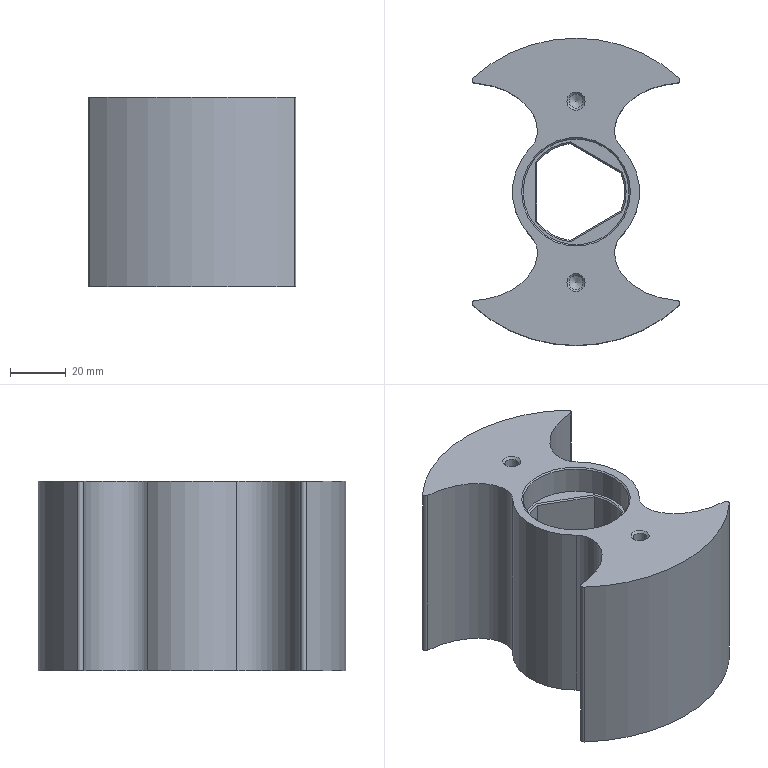Part | 1 solid | 50 faces | box 74.46 x 110.159 x 68 mm | volume 259040 mm3 | cylinder 17 | cone 16 | plane 13 | spline 4 | commonest cylinder face diameters 2.25 x4 35 x3 2.5 x2 5 x2 45.541 x2 110.159 x2
STEP:
#1=CARTESIAN_POINT('',(-1.35,20.25,-68.));
#2=VERTEX_POINT('',#1);
#3=CARTESIAN_POINT('',(0.,20.25,-68.));
#4=DIRECTION('',(0.,0.,-1.));
#5=DIRECTION('',(-1.,0.,0.));
#6=AXIS2_PLACEMENT_3D('',#3,#4,#5);
#7=CIRCLE('',#6,1.35);
#8=EDGE_CURVE('',#2,#2,#7,.T.);
#9=ORIENTED_EDGE('',*,*,#8,.F.);
#10=EDGE_LOOP('',(#9));
#11=FACE_BOUND('',#10,.T.);
#12=CARTESIAN_POINT('',(18.8,0.,-68.));
#13=VERTEX_POINT('',#12);
#14=CARTESIAN_POINT('',(0.,0.,-68.));
#15=DIRECTION('',(0.,0.,1.));
#16=DIRECTION('',(1.,0.,0.));
#17=AXIS2_PLACEMENT_3D('',#14,#15,#16);
#18=CIRCLE('',#17,18.8);
#19=EDGE_CURVE('',#13,#13,#18,.T.);
#20=ORIENTED_EDGE('',*,*,#19,.T.);
#21=EDGE_LOOP('',(#20));
#22=FACE_BOUND('',#21,.T.);
#23=CARTESIAN_POINT('',(-36.858,-40.93,-68.));
#24=VERTEX_POINT('',#23);
#25=CARTESIAN_POINT('',(36.858,-40.93,-68.));
#26=VERTEX_POINT('',#25);
#27=CARTESIAN_POINT('',(0.,0.,-68.));
#28=DIRECTION('',(0.,0.,1.));
#29=DIRECTION('',(1.,0.,0.));
#30=AXIS2_PLACEMENT_3D('',#27,#28,#29);
#31=CIRCLE('',#30,55.079);
#32=EDGE_CURVE('',#24,#26,#31,.T.);
#33=ORIENTED_EDGE('',*,*,#32,.F.);
#34=CARTESIAN_POINT('',(-36.188,-38.972,-68.));
#35=VERTEX_POINT('',#34);
#36=CARTESIAN_POINT('',(-36.105,-40.094,-68.));
#37=DIRECTION('',(0.,0.,1.));
#38=DIRECTION('',(1.,0.,0.));
#39=AXIS2_PLACEMENT_3D('',#36,#37,#38);
#40=CIRCLE('',#39,1.125);
#41=EDGE_CURVE('',#35,#24,#40,.T.);
#42=ORIENTED_EDGE('',*,*,#41,.F.);
#43=CARTESIAN_POINT('',(-16.101,-16.101,-68.));
#44=VERTEX_POINT('',#43);
#45=CARTESIAN_POINT('',(-16.101,-16.101,-68.));
#46=CARTESIAN_POINT('',(-14.995,-17.215,-68.));
#47=CARTESIAN_POINT('',(-13.563,-20.098,-68.));
#48=CARTESIAN_POINT('',(-13.933,-24.897,-68.));
#49=CARTESIAN_POINT('',(-16.007,-29.108,-68.));
#50=CARTESIAN_POINT('',(-20.192,-33.725,-68.));
#51=CARTESIAN_POINT('',(-27.057,-37.533,-68.));
#52=CARTESIAN_POINT('',(-33.099,-38.735,-68.));
#53=CARTESIAN_POINT('',(-36.188,-38.972,-68.));
#54=B_SPLINE_CURVE_WITH_KNOTS('',3,(#45,#46,#47,#48,#49,#50,#51,#52,#53),.UNSPECIFIED.,.F.,.F.,(4,1,1,1,1,1,4),(0.,0.004639,0.009278,0.01392,0.01856,0.02783,0.03711),.UNSPECIFIED.);
#55=EDGE_CURVE('',#44,#35,#54,.T.);
#56=ORIENTED_EDGE('',*,*,#55,.F.);
#57=CARTESIAN_POINT('',(-16.101,16.101,-68.));
#58=VERTEX_POINT('',#57);
#59=CARTESIAN_POINT('',(0.,0.,-68.));
#60=DIRECTION('',(0.,0.,1.));
#61=DIRECTION('',(1.,0.,0.));
#62=AXIS2_PLACEMENT_3D('',#59,#60,#61);
#63=CIRCLE('',#62,22.771);
#64=EDGE_CURVE('',#58,#44,#63,.T.);
#65=ORIENTED_EDGE('',*,*,#64,.F.);
#66=CARTESIAN_POINT('',(-36.188,38.972,-68.));
#67=VERTEX_POINT('',#66);
#68=CARTESIAN_POINT('',(-36.188,38.972,-68.));
#69=CARTESIAN_POINT('',(-33.1,38.735,-68.));
#70=CARTESIAN_POINT('',(-27.074,37.541,-68.));
#71=CARTESIAN_POINT('',(-20.182,33.717,-68.));
#72=CARTESIAN_POINT('',(-16.008,29.109,-68.));
#73=CARTESIAN_POINT('',(-13.931,24.889,-68.));
#74=CARTESIAN_POINT('',(-13.564,20.1,-68.));
#75=CARTESIAN_POINT('',(-14.995,17.216,-68.));
#76=CARTESIAN_POINT('',(-16.101,16.101,-68.));
#77=B_SPLINE_CURVE_WITH_KNOTS('',3,(#68,#69,#70,#71,#72,#73,#74,#75,#76),.UNSPECIFIED.,.F.,.F.,(4,1,1,1,1,1,4),(0.,0.009182,0.01836,0.02295,0.02755,0.03214,0.03673),.UNSPECIFIED.);
#78=EDGE_CURVE('',#67,#58,#77,.T.);
#79=ORIENTED_EDGE('',*,*,#78,.F.);
#80=CARTESIAN_POINT('',(-36.858,40.93,-68.));
#81=VERTEX_POINT('',#80);
#82=CARTESIAN_POINT('',(-36.105,40.094,-68.));
#83=DIRECTION('',(0.,0.,1.));
#84=DIRECTION('',(1.,0.,0.));
#85=AXIS2_PLACEMENT_3D('',#82,#83,#84);
#86=CIRCLE('',#85,1.125);
#87=EDGE_CURVE('',#81,#67,#86,.T.);
#88=ORIENTED_EDGE('',*,*,#87,.F.);
#89=CARTESIAN_POINT('',(36.858,40.93,-68.));
#90=VERTEX_POINT('',#89);
#91=CARTESIAN_POINT('',(0.,0.,-68.));
#92=DIRECTION('',(0.,0.,1.));
#93=DIRECTION('',(1.,0.,0.));
#94=AXIS2_PLACEMENT_3D('',#91,#92,#93);
#95=CIRCLE('',#94,55.079);
#96=EDGE_CURVE('',#90,#81,#95,.T.);
#97=ORIENTED_EDGE('',*,*,#96,.F.);
#98=CARTESIAN_POINT('',(36.188,38.972,-68.));
#99=VERTEX_POINT('',#98);
#100=CARTESIAN_POINT('',(36.105,40.094,-68.));
#101=DIRECTION('',(0.,0.,1.));
#102=DIRECTION('',(1.,0.,0.));
#103=AXIS2_PLACEMENT_3D('',#100,#101,#102);
#104=CIRCLE('',#103,1.125);
#105=EDGE_CURVE('',#99,#90,#104,.T.);
#106=ORIENTED_EDGE('',*,*,#105,.F.);
#107=CARTESIAN_POINT('',(16.101,16.101,-68.));
#108=VERTEX_POINT('',#107);
#109=CARTESIAN_POINT('',(16.101,16.101,-68.));
#110=CARTESIAN_POINT('',(14.995,17.215,-68.));
#111=CARTESIAN_POINT('',(13.563,20.098,-68.));
#112=CARTESIAN_POINT('',(13.933,24.897,-68.));
#113=CARTESIAN_POINT('',(16.007,29.108,-68.));
#114=CARTESIAN_POINT('',(20.192,33.725,-68.));
#115=CARTESIAN_POINT('',(27.057,37.533,-68.));
#116=CARTESIAN_POINT('',(33.099,38.735,-68.));
#117=CARTESIAN_POINT('',(36.188,38.972,-68.));
#118=B_SPLINE_CURVE_WITH_KNOTS('',3,(#109,#110,#111,#112,#113,#114,#115,#116,#117),.UNSPECIFIED.,.F.,.F.,(4,1,1,1,1,1,4),(0.,0.004639,0.009278,0.01392,0.01856,0.02783,0.03711),.UNSPECIFIED.);
#119=EDGE_CURVE('',#108,#99,#118,.T.);
#120=ORIENTED_EDGE('',*,*,#119,.F.);
#121=CARTESIAN_POINT('',(16.101,-16.101,-68.));
#122=VERTEX_POINT('',#121);
#123=CARTESIAN_POINT('',(0.,0.,-68.));
#124=DIRECTION('',(0.,0.,1.));
#125=DIRECTION('',(1.,0.,0.));
#126=AXIS2_PLACEMENT_3D('',#123,#124,#125);
#127=CIRCLE('',#126,22.771);
#128=EDGE_CURVE('',#122,#108,#127,.T.);
#129=ORIENTED_EDGE('',*,*,#128,.F.);
#130=CARTESIAN_POINT('',(36.188,-38.972,-68.));
#131=VERTEX_POINT('',#130);
#132=CARTESIAN_POINT('',(36.188,-38.972,-68.));
#133=CARTESIAN_POINT('',(33.1,-38.735,-68.));
#134=CARTESIAN_POINT('',(27.074,-37.541,-68.));
#135=CARTESIAN_POINT('',(20.182,-33.717,-68.));
#136=CARTESIAN_POINT('',(16.008,-29.109,-68.));
#137=CARTESIAN_POINT('',(13.931,-24.889,-68.));
#138=CARTESIAN_POINT('',(13.564,-20.1,-68.));
#139=CARTESIAN_POINT('',(14.995,-17.216,-68.));
#140=CARTESIAN_POINT('',(16.101,-16.101,-68.));
#141=B_SPLINE_CURVE_WITH_KNOTS('',3,(#132,#133,#134,#135,#136,#137,#138,#139,#140),.UNSPECIFIED.,.F.,.F.,(4,1,1,1,1,1,4),(0.,0.009182,0.01836,0.02295,0.02755,0.03214,0.03673),.UNSPECIFIED.);
#142=EDGE_CURVE('',#131,#122,#141,.T.);
#143=ORIENTED_EDGE('',*,*,#142,.F.);
#144=CARTESIAN_POINT('',(36.105,-40.094,-68.));
#145=DIRECTION('',(0.,0.,1.));
#146=DIRECTION('',(1.,0.,0.));
#147=AXIS2_PLACEMENT_3D('',#144,#145,#146);
#148=CIRCLE('',#147,1.125);
#149=EDGE_CURVE('',#26,#131,#148,.T.);
#150=ORIENTED_EDGE('',*,*,#149,.F.);
#151=EDGE_LOOP('',(#33,#42,#56,#65,#79,#88,#97,#106,#120,#129,#143,#150));
#152=FACE_BOUND('',#151,.T.);
#153=CARTESIAN_POINT('',(-1.35,-20.25,-68.));
#154=VERTEX_POINT('',#153);
#155=CARTESIAN_POINT('',(0.,-20.25,-68.));
#156=DIRECTION('',(0.,0.,-1.));
#157=DIRECTION('',(-1.,0.,0.));
#158=AXIS2_PLACEMENT_3D('',#155,#156,#157);
#159=CIRCLE('',#158,1.35);
#160=EDGE_CURVE('',#154,#154,#159,.T.);
#161=ORIENTED_EDGE('',*,*,#160,.F.);
#162=EDGE_LOOP('',(#161));
#163=FACE_BOUND('',#162,.T.);
#164=CARTESIAN_POINT('',(0.,0.,-68.));
#165=DIRECTION('',(0.,0.,1.));
#166=DIRECTION('',(1.,0.,0.));
#167=AXIS2_PLACEMENT_3D('',#164,#165,#166);
#168=PLANE('',#167);
#169=ADVANCED_FACE('',(#11,#22,#152,#163),#168,.F.);
#170=CARTESIAN_POINT('',(-2.093,17.374,-10.7));
#171=VERTEX_POINT('',#170);
#172=CARTESIAN_POINT('',(-2.093,17.374,-62.5));
#173=VERTEX_POINT('',#172);
#174=CARTESIAN_POINT('',(-2.093,17.374,11.09));
#175=DIRECTION('',(0.,0.,-1.));
#176=VECTOR('',#175,1000.);
#177=LINE('',#174,#176);
#178=EDGE_CURVE('',#171,#173,#177,.T.);
#179=ORIENTED_EDGE('',*,*,#178,.F.);
#180=CARTESIAN_POINT('',(-14.,10.5,-10.7));
#181=VERTEX_POINT('',#180);
#182=CARTESIAN_POINT('',(0.,0.,-10.7));
#183=DIRECTION('',(0.,0.,-1.));
#184=DIRECTION('',(-1.,0.,0.));
#185=AXIS2_PLACEMENT_3D('',#182,#183,#184);
#186=CIRCLE('',#185,17.5);
#187=EDGE_CURVE('',#171,#181,#186,.F.);
#188=ORIENTED_EDGE('',*,*,#187,.T.);
#189=CARTESIAN_POINT('',(-14.,10.5,-62.5));
#190=VERTEX_POINT('',#189);
#191=CARTESIAN_POINT('',(-14.,10.5,11.09));
#192=DIRECTION('',(0.,0.,-1.));
#193=VECTOR('',#192,1000.);
#194=LINE('',#191,#193);
#195=EDGE_CURVE('',#181,#190,#194,.T.);
#196=ORIENTED_EDGE('',*,*,#195,.T.);
#197=CARTESIAN_POINT('',(0.,0.,-62.5));
#198=DIRECTION('',(0.,0.,1.));
#199=DIRECTION('',(1.,0.,0.));
#200=AXIS2_PLACEMENT_3D('',#197,#198,#199);
#201=CIRCLE('',#200,17.5);
#202=EDGE_CURVE('',#190,#173,#201,.F.);
#203=ORIENTED_EDGE('',*,*,#202,.T.);
#204=EDGE_LOOP('',(#179,#188,#196,#203));
#205=FACE_BOUND('',#204,.T.);
#206=CARTESIAN_POINT('',(0.,0.,-68.));
#207=DIRECTION('',(0.,0.,-1.));
#208=DIRECTION('',(-1.,0.,0.));
#209=AXIS2_PLACEMENT_3D('',#206,#207,#208);
#210=CYLINDRICAL_SURFACE('',#209,17.5);
#211=ADVANCED_FACE('',(#205),#210,.F.);
#212=CARTESIAN_POINT('',(16.093,-6.874,-10.7));
#213=VERTEX_POINT('',#212);
#214=CARTESIAN_POINT('',(16.093,-6.874,-62.5));
#215=VERTEX_POINT('',#214);
#216=CARTESIAN_POINT('',(16.093,-6.874,11.09));
#217=DIRECTION('',(0.,0.,-1.));
#218=VECTOR('',#217,1000.);
#219=LINE('',#216,#218);
#220=EDGE_CURVE('',#213,#215,#219,.T.);
#221=ORIENTED_EDGE('',*,*,#220,.F.);
#222=CARTESIAN_POINT('',(16.093,6.874,-10.7));
#223=VERTEX_POINT('',#222);
#224=CARTESIAN_POINT('',(0.,0.,-10.7));
#225=DIRECTION('',(0.,0.,-1.));
#226=DIRECTION('',(-1.,0.,0.));
#227=AXIS2_PLACEMENT_3D('',#224,#225,#226);
#228=CIRCLE('',#227,17.5);
#229=EDGE_CURVE('',#213,#223,#228,.F.);
#230=ORIENTED_EDGE('',*,*,#229,.T.);
#231=CARTESIAN_POINT('',(16.093,6.874,-62.5));
#232=VERTEX_POINT('',#231);
#233=CARTESIAN_POINT('',(16.093,6.874,11.09));
#234=DIRECTION('',(0.,0.,-1.));
#235=VECTOR('',#234,1000.);
#236=LINE('',#233,#235);
#237=EDGE_CURVE('',#223,#232,#236,.T.);
#238=ORIENTED_EDGE('',*,*,#237,.T.);
#239=CARTESIAN_POINT('',(0.,0.,-62.5));
#240=DIRECTION('',(0.,0.,1.));
#241=DIRECTION('',(1.,0.,0.));
#242=AXIS2_PLACEMENT_3D('',#239,#240,#241);
#243=CIRCLE('',#242,17.5);
#244=EDGE_CURVE('',#232,#215,#243,.F.);
#245=ORIENTED_EDGE('',*,*,#244,.T.);
#246=EDGE_LOOP('',(#221,#230,#238,#245));
#247=FACE_BOUND('',#246,.T.);
#248=CARTESIAN_POINT('',(0.,0.,-68.));
#249=DIRECTION('',(0.,0.,-1.));
#250=DIRECTION('',(-1.,0.,0.));
#251=AXIS2_PLACEMENT_3D('',#248,#249,#250);
#252=CYLINDRICAL_SURFACE('',#251,17.5);
#253=ADVANCED_FACE('',(#247),#252,.F.);
#254=ORIENTED_EDGE('',*,*,#32,.T.);
#255=CARTESIAN_POINT('',(36.858,-40.93,0.));
#256=VERTEX_POINT('',#255);
#257=CARTESIAN_POINT('',(36.858,-40.93,0.));
#258=DIRECTION('',(0.,0.,-1.));
#259=VECTOR('',#258,1000.);
#260=LINE('',#257,#259);
#261=EDGE_CURVE('',#256,#26,#260,.T.);
#262=ORIENTED_EDGE('',*,*,#261,.F.);
#263=CARTESIAN_POINT('',(-36.858,-40.93,0.));
#264=VERTEX_POINT('',#263);
#265=CARTESIAN_POINT('',(0.,0.,0.));
#266=DIRECTION('',(0.,0.,1.));
#267=DIRECTION('',(1.,0.,0.));
#268=AXIS2_PLACEMENT_3D('',#265,#266,#267);
#269=CIRCLE('',#268,55.079);
#270=EDGE_CURVE('',#264,#256,#269,.T.);
#271=ORIENTED_EDGE('',*,*,#270,.F.);
#272=CARTESIAN_POINT('',(-36.858,-40.93,0.));
#273=DIRECTION('',(0.,0.,-1.));
#274=VECTOR('',#273,1000.);
#275=LINE('',#272,#274);
#276=EDGE_CURVE('',#264,#24,#275,.T.);
#277=ORIENTED_EDGE('',*,*,#276,.T.);
#278=EDGE_LOOP('',(#254,#262,#271,#277));
#279=FACE_BOUND('',#278,.T.);
#280=CARTESIAN_POINT('',(0.,0.,0.));
#281=DIRECTION('',(0.,0.,-1.));
#282=DIRECTION('',(-1.,0.,0.));
#283=AXIS2_PLACEMENT_3D('',#280,#281,#282);
#284=CYLINDRICAL_SURFACE('',#283,55.079);
#285=ADVANCED_FACE('',(#279),#284,.T.);
#286=ORIENTED_EDGE('',*,*,#149,.T.);
#287=CARTESIAN_POINT('',(36.188,-38.972,0.));
#288=VERTEX_POINT('',#287);
#289=CARTESIAN_POINT('',(36.188,-38.972,0.));
#290=DIRECTION('',(0.,0.,-1.));
#291=VECTOR('',#290,1000.);
#292=LINE('',#289,#291);
#293=EDGE_CURVE('',#288,#131,#292,.T.);
#294=ORIENTED_EDGE('',*,*,#293,.F.);
#295=CARTESIAN_POINT('',(36.105,-40.094,0.));
#296=DIRECTION('',(0.,0.,1.));
#297=DIRECTION('',(1.,0.,0.));
#298=AXIS2_PLACEMENT_3D('',#295,#296,#297);
#299=CIRCLE('',#298,1.125);
#300=EDGE_CURVE('',#256,#288,#299,.T.);
#301=ORIENTED_EDGE('',*,*,#300,.F.);
#302=ORIENTED_EDGE('',*,*,#261,.T.);
#303=EDGE_LOOP('',(#286,#294,#301,#302));
#304=FACE_BOUND('',#303,.T.);
#305=CARTESIAN_POINT('',(36.105,-40.094,0.));
#306=DIRECTION('',(0.,0.,-1.));
#307=DIRECTION('',(-1.,0.,0.));
#308=AXIS2_PLACEMENT_3D('',#305,#306,#307);
#309=CYLINDRICAL_SURFACE('',#308,1.125);
#310=ADVANCED_FACE('',(#304),#309,.T.);
#311=ORIENTED_EDGE('',*,*,#142,.T.);
#312=CARTESIAN_POINT('',(16.101,-16.101,0.));
#313=VERTEX_POINT('',#312);
#314=CARTESIAN_POINT('',(16.101,-16.101,0.));
#315=DIRECTION('',(0.,0.,-1.));
#316=VECTOR('',#315,1000.);
#317=LINE('',#314,#316);
#318=EDGE_CURVE('',#313,#122,#317,.T.);
#319=ORIENTED_EDGE('',*,*,#318,.F.);
#320=CARTESIAN_POINT('',(36.188,-38.972,0.));
#321=CARTESIAN_POINT('',(33.1,-38.735,0.));
#322=CARTESIAN_POINT('',(27.074,-37.541,0.));
#323=CARTESIAN_POINT('',(20.182,-33.717,0.));
#324=CARTESIAN_POINT('',(16.008,-29.109,0.));
#325=CARTESIAN_POINT('',(13.931,-24.889,0.));
#326=CARTESIAN_POINT('',(13.564,-20.1,0.));
#327=CARTESIAN_POINT('',(14.995,-17.216,0.));
#328=CARTESIAN_POINT('',(16.101,-16.101,0.));
#329=B_SPLINE_CURVE_WITH_KNOTS('',3,(#320,#321,#322,#323,#324,#325,#326,#327,#328),.UNSPECIFIED.,.F.,.F.,(4,1,1,1,1,1,4),(0.,0.009182,0.01836,0.02295,0.02755,0.03214,0.03673),.UNSPECIFIED.);
#330=EDGE_CURVE('',#288,#313,#329,.T.);
#331=ORIENTED_EDGE('',*,*,#330,.F.);
#332=ORIENTED_EDGE('',*,*,#293,.T.);
#333=EDGE_LOOP('',(#311,#319,#331,#332));
#334=FACE_BOUND('',#333,.T.);
#335=CARTESIAN_POINT('',(36.188,-38.972,0.));
#336=CARTESIAN_POINT('',(36.188,-38.972,-68.));
#337=CARTESIAN_POINT('',(33.121,-38.737,0.));
#338=CARTESIAN_POINT('',(33.121,-38.737,-68.));
#339=CARTESIAN_POINT('',(27.013,-37.524,0.));
#340=CARTESIAN_POINT('',(27.013,-37.524,-68.));
#341=CARTESIAN_POINT('',(20.163,-33.701,0.));
#342=CARTESIAN_POINT('',(20.163,-33.701,-68.));
#343=CARTESIAN_POINT('',(15.987,-29.082,0.));
#344=CARTESIAN_POINT('',(15.987,-29.082,-68.));
#345=CARTESIAN_POINT('',(13.93,-24.864,0.));
#346=CARTESIAN_POINT('',(13.93,-24.864,-68.));
#347=CARTESIAN_POINT('',(13.556,-20.109,0.));
#348=CARTESIAN_POINT('',(13.556,-20.109,-68.));
#349=CARTESIAN_POINT('',(15.018,-17.192,0.));
#350=CARTESIAN_POINT('',(15.018,-17.192,-68.));
#351=CARTESIAN_POINT('',(16.101,-16.101,0.));
#352=CARTESIAN_POINT('',(16.101,-16.101,-68.));
#353=B_SPLINE_SURFACE_WITH_KNOTS('',3,1,((#335,#336),(#337,#338),(#339,#340),(#341,#342),(#343,#344),(#345,#346),(#347,#348),(#349,#350),(#351,#352)),.SURF_OF_LINEAR_EXTRUSION.,.F.,.F.,.F.,(4,1,1,1,1,1,4),(2,2),(0.,0.25,0.5,0.625,0.75,0.875,1.),(0.,1.),.UNSPECIFIED.);
#354=ADVANCED_FACE('',(#334),#353,.F.);
#355=ORIENTED_EDGE('',*,*,#128,.T.);
#356=CARTESIAN_POINT('',(16.101,16.101,0.));
#357=VERTEX_POINT('',#356);
#358=CARTESIAN_POINT('',(16.101,16.101,0.));
#359=DIRECTION('',(0.,0.,-1.));
#360=VECTOR('',#359,1000.);
#361=LINE('',#358,#360);
#362=EDGE_CURVE('',#357,#108,#361,.T.);
#363=ORIENTED_EDGE('',*,*,#362,.F.);
#364=CARTESIAN_POINT('',(0.,0.,0.));
#365=DIRECTION('',(0.,0.,1.));
#366=DIRECTION('',(1.,0.,0.));
#367=AXIS2_PLACEMENT_3D('',#364,#365,#366);
#368=CIRCLE('',#367,22.771);
#369=EDGE_CURVE('',#313,#357,#368,.T.);
#370=ORIENTED_EDGE('',*,*,#369,.F.);
#371=ORIENTED_EDGE('',*,*,#318,.T.);
#372=EDGE_LOOP('',(#355,#363,#370,#371));
#373=FACE_BOUND('',#372,.T.);
#374=CARTESIAN_POINT('',(0.,0.,0.));
#375=DIRECTION('',(0.,0.,-1.));
#376=DIRECTION('',(-1.,0.,0.));
#377=AXIS2_PLACEMENT_3D('',#374,#375,#376);
#378=CYLINDRICAL_SURFACE('',#377,22.771);
#379=ADVANCED_FACE('',(#373),#378,.T.);
#380=ORIENTED_EDGE('',*,*,#119,.T.);
#381=CARTESIAN_POINT('',(36.188,38.972,0.));
#382=VERTEX_POINT('',#381);
#383=CARTESIAN_POINT('',(36.188,38.972,0.));
#384=DIRECTION('',(0.,0.,-1.));
#385=VECTOR('',#384,1000.);
#386=LINE('',#383,#385);
#387=EDGE_CURVE('',#382,#99,#386,.T.);
#388=ORIENTED_EDGE('',*,*,#387,.F.);
#389=CARTESIAN_POINT('',(16.101,16.101,0.));
#390=CARTESIAN_POINT('',(14.995,17.215,0.));
#391=CARTESIAN_POINT('',(13.563,20.098,0.));
#392=CARTESIAN_POINT('',(13.933,24.897,0.));
#393=CARTESIAN_POINT('',(16.007,29.108,0.));
#394=CARTESIAN_POINT('',(20.192,33.725,0.));
#395=CARTESIAN_POINT('',(27.057,37.533,0.));
#396=CARTESIAN_POINT('',(33.099,38.735,0.));
#397=CARTESIAN_POINT('',(36.188,38.972,0.));
#398=B_SPLINE_CURVE_WITH_KNOTS('',3,(#389,#390,#391,#392,#393,#394,#395,#396,#397),.UNSPECIFIED.,.F.,.F.,(4,1,1,1,1,1,4),(0.,0.004639,0.009278,0.01392,0.01856,0.02783,0.03711),.UNSPECIFIED.);
#399=EDGE_CURVE('',#357,#382,#398,.T.);
#400=ORIENTED_EDGE('',*,*,#399,.F.);
#401=ORIENTED_EDGE('',*,*,#362,.T.);
#402=EDGE_LOOP('',(#380,#388,#400,#401));
#403=FACE_BOUND('',#402,.T.);
#404=CARTESIAN_POINT('',(16.101,16.101,0.));
#405=CARTESIAN_POINT('',(16.101,16.101,-68.));
#406=CARTESIAN_POINT('',(15.018,17.192,0.));
#407=CARTESIAN_POINT('',(15.018,17.192,-68.));
#408=CARTESIAN_POINT('',(13.556,20.109,0.));
#409=CARTESIAN_POINT('',(13.556,20.109,-68.));
#410=CARTESIAN_POINT('',(13.93,24.864,0.));
#411=CARTESIAN_POINT('',(13.93,24.864,-68.));
#412=CARTESIAN_POINT('',(15.987,29.083,0.));
#413=CARTESIAN_POINT('',(15.987,29.083,-68.));
#414=CARTESIAN_POINT('',(20.163,33.702,0.));
#415=CARTESIAN_POINT('',(20.163,33.702,-68.));
#416=CARTESIAN_POINT('',(27.014,37.524,0.));
#417=CARTESIAN_POINT('',(27.014,37.524,-68.));
#418=CARTESIAN_POINT('',(33.122,38.737,0.));
#419=CARTESIAN_POINT('',(33.122,38.737,-68.));
#420=CARTESIAN_POINT('',(36.188,38.972,0.));
#421=CARTESIAN_POINT('',(36.188,38.972,-68.));
#422=B_SPLINE_SURFACE_WITH_KNOTS('',3,1,((#404,#405),(#406,#407),(#408,#409),(#410,#411),(#412,#413),(#414,#415),(#416,#417),(#418,#419),(#420,#421)),.SURF_OF_LINEAR_EXTRUSION.,.F.,.F.,.F.,(4,1,1,1,1,1,4),(2,2),(-0.000003449,0.125,0.25,0.375,0.5,0.75,1.),(0.,1.),.UNSPECIFIED.);
#423=ADVANCED_FACE('',(#403),#422,.F.);
#424=ORIENTED_EDGE('',*,*,#105,.T.);
#425=CARTESIAN_POINT('',(36.858,40.93,0.));
#426=VERTEX_POINT('',#425);
#427=CARTESIAN_POINT('',(36.858,40.93,0.));
#428=DIRECTION('',(0.,0.,-1.));
#429=VECTOR('',#428,1000.);
#430=LINE('',#427,#429);
#431=EDGE_CURVE('',#426,#90,#430,.T.);
#432=ORIENTED_EDGE('',*,*,#431,.F.);
#433=CARTESIAN_POINT('',(36.105,40.094,0.));
#434=DIRECTION('',(0.,0.,1.));
#435=DIRECTION('',(1.,0.,0.));
#436=AXIS2_PLACEMENT_3D('',#433,#434,#435);
#437=CIRCLE('',#436,1.125);
#438=EDGE_CURVE('',#382,#426,#437,.T.);
#439=ORIENTED_EDGE('',*,*,#438,.F.);
#440=ORIENTED_EDGE('',*,*,#387,.T.);
#441=EDGE_LOOP('',(#424,#432,#439,#440));
#442=FACE_BOUND('',#441,.T.);
#443=CARTESIAN_POINT('',(36.105,40.094,0.));
#444=DIRECTION('',(0.,0.,-1.));
#445=DIRECTION('',(-1.,0.,0.));
#446=AXIS2_PLACEMENT_3D('',#443,#444,#445);
#447=CYLINDRICAL_SURFACE('',#446,1.125);
#448=ADVANCED_FACE('',(#442),#447,.T.);
#449=ORIENTED_EDGE('',*,*,#96,.T.);
#450=CARTESIAN_POINT('',(-36.858,40.93,0.));
#451=VERTEX_POINT('',#450);
#452=CARTESIAN_POINT('',(-36.858,40.93,0.));
#453=DIRECTION('',(0.,0.,-1.));
#454=VECTOR('',#453,1000.);
#455=LINE('',#452,#454);
#456=EDGE_CURVE('',#451,#81,#455,.T.);
#457=ORIENTED_EDGE('',*,*,#456,.F.);
#458=CARTESIAN_POINT('',(0.,0.,0.));
#459=DIRECTION('',(0.,0.,1.));
#460=DIRECTION('',(1.,0.,0.));
#461=AXIS2_PLACEMENT_3D('',#458,#459,#460);
#462=CIRCLE('',#461,55.079);
#463=EDGE_CURVE('',#426,#451,#462,.T.);
#464=ORIENTED_EDGE('',*,*,#463,.F.);
#465=ORIENTED_EDGE('',*,*,#431,.T.);
#466=EDGE_LOOP('',(#449,#457,#464,#465));
#467=FACE_BOUND('',#466,.T.);
#468=CARTESIAN_POINT('',(0.,0.,0.));
#469=DIRECTION('',(0.,0.,-1.));
#470=DIRECTION('',(-1.,0.,0.));
#471=AXIS2_PLACEMENT_3D('',#468,#469,#470);
#472=CYLINDRICAL_SURFACE('',#471,55.079);
#473=ADVANCED_FACE('',(#467),#472,.T.);
#474=ORIENTED_EDGE('',*,*,#87,.T.);
#475=CARTESIAN_POINT('',(-36.188,38.972,0.));
#476=VERTEX_POINT('',#475);
#477=CARTESIAN_POINT('',(-36.188,38.972,0.));
#478=DIRECTION('',(0.,0.,-1.));
#479=VECTOR('',#478,1000.);
#480=LINE('',#477,#479);
#481=EDGE_CURVE('',#476,#67,#480,.T.);
#482=ORIENTED_EDGE('',*,*,#481,.F.);
#483=CARTESIAN_POINT('',(-36.105,40.094,0.));
#484=DIRECTION('',(0.,0.,1.));
#485=DIRECTION('',(1.,0.,0.));
#486=AXIS2_PLACEMENT_3D('',#483,#484,#485);
#487=CIRCLE('',#486,1.125);
#488=EDGE_CURVE('',#451,#476,#487,.T.);
#489=ORIENTED_EDGE('',*,*,#488,.F.);
#490=ORIENTED_EDGE('',*,*,#456,.T.);
#491=EDGE_LOOP('',(#474,#482,#489,#490));
#492=FACE_BOUND('',#491,.T.);
#493=CARTESIAN_POINT('',(-36.105,40.094,0.));
#494=DIRECTION('',(0.,0.,-1.));
#495=DIRECTION('',(-1.,0.,0.));
#496=AXIS2_PLACEMENT_3D('',#493,#494,#495);
#497=CYLINDRICAL_SURFACE('',#496,1.125);
#498=ADVANCED_FACE('',(#492),#497,.T.);
#499=ORIENTED_EDGE('',*,*,#78,.T.);
#500=CARTESIAN_POINT('',(-16.101,16.101,0.));
#501=VERTEX_POINT('',#500);
#502=CARTESIAN_POINT('',(-16.101,16.101,0.));
#503=DIRECTION('',(0.,0.,-1.));
#504=VECTOR('',#503,1000.);
#505=LINE('',#502,#504);
#506=EDGE_CURVE('',#501,#58,#505,.T.);
#507=ORIENTED_EDGE('',*,*,#506,.F.);
#508=CARTESIAN_POINT('',(-36.188,38.972,0.));
#509=CARTESIAN_POINT('',(-33.1,38.735,0.));
#510=CARTESIAN_POINT('',(-27.074,37.541,0.));
#511=CARTESIAN_POINT('',(-20.182,33.717,0.));
#512=CARTESIAN_POINT('',(-16.008,29.109,0.));
#513=CARTESIAN_POINT('',(-13.931,24.889,0.));
#514=CARTESIAN_POINT('',(-13.564,20.1,0.));
#515=CARTESIAN_POINT('',(-14.995,17.216,0.));
#516=CARTESIAN_POINT('',(-16.101,16.101,0.));
#517=B_SPLINE_CURVE_WITH_KNOTS('',3,(#508,#509,#510,#511,#512,#513,#514,#515,#516),.UNSPECIFIED.,.F.,.F.,(4,1,1,1,1,1,4),(0.,0.009182,0.01836,0.02295,0.02755,0.03214,0.03673),.UNSPECIFIED.);
#518=EDGE_CURVE('',#476,#501,#517,.T.);
#519=ORIENTED_EDGE('',*,*,#518,.F.);
#520=ORIENTED_EDGE('',*,*,#481,.T.);
#521=EDGE_LOOP('',(#499,#507,#519,#520));
#522=FACE_BOUND('',#521,.T.);
#523=CARTESIAN_POINT('',(-36.188,38.972,0.));
#524=CARTESIAN_POINT('',(-36.188,38.972,-68.));
#525=CARTESIAN_POINT('',(-33.121,38.737,0.));
#526=CARTESIAN_POINT('',(-33.121,38.737,-68.));
#527=CARTESIAN_POINT('',(-27.013,37.524,0.));
#528=CARTESIAN_POINT('',(-27.013,37.524,-68.));
#529=CARTESIAN_POINT('',(-20.163,33.701,0.));
#530=CARTESIAN_POINT('',(-20.163,33.701,-68.));
#531=CARTESIAN_POINT('',(-15.987,29.082,0.));
#532=CARTESIAN_POINT('',(-15.987,29.082,-68.));
#533=CARTESIAN_POINT('',(-13.93,24.864,0.));
#534=CARTESIAN_POINT('',(-13.93,24.864,-68.));
#535=CARTESIAN_POINT('',(-13.556,20.109,0.));
#536=CARTESIAN_POINT('',(-13.556,20.109,-68.));
#537=CARTESIAN_POINT('',(-15.018,17.192,0.));
#538=CARTESIAN_POINT('',(-15.018,17.192,-68.));
#539=CARTESIAN_POINT('',(-16.101,16.101,0.));
#540=CARTESIAN_POINT('',(-16.101,16.101,-68.));
#541=B_SPLINE_SURFACE_WITH_KNOTS('',3,1,((#523,#524),(#525,#526),(#527,#528),(#529,#530),(#531,#532),(#533,#534),(#535,#536),(#537,#538),(#539,#540)),.SURF_OF_LINEAR_EXTRUSION.,.F.,.F.,.F.,(4,1,1,1,1,1,4),(2,2),(0.,0.25,0.5,0.625,0.75,0.875,1.),(0.,1.),.UNSPECIFIED.);
#542=ADVANCED_FACE('',(#522),#541,.F.);
#543=ORIENTED_EDGE('',*,*,#64,.T.);
#544=CARTESIAN_POINT('',(-16.101,-16.101,0.));
#545=VERTEX_POINT('',#544);
#546=CARTESIAN_POINT('',(-16.101,-16.101,0.));
#547=DIRECTION('',(0.,0.,-1.));
#548=VECTOR('',#547,1000.);
#549=LINE('',#546,#548);
#550=EDGE_CURVE('',#545,#44,#549,.T.);
#551=ORIENTED_EDGE('',*,*,#550,.F.);
#552=CARTESIAN_POINT('',(0.,0.,0.));
#553=DIRECTION('',(0.,0.,1.));
#554=DIRECTION('',(1.,0.,0.));
#555=AXIS2_PLACEMENT_3D('',#552,#553,#554);
#556=CIRCLE('',#555,22.771);
#557=EDGE_CURVE('',#501,#545,#556,.T.);
#558=ORIENTED_EDGE('',*,*,#557,.F.);
#559=ORIENTED_EDGE('',*,*,#506,.T.);
#560=EDGE_LOOP('',(#543,#551,#558,#559));
#561=FACE_BOUND('',#560,.T.);
#562=CARTESIAN_POINT('',(0.,0.,0.));
#563=DIRECTION('',(0.,0.,-1.));
#564=DIRECTION('',(-1.,0.,0.));
#565=AXIS2_PLACEMENT_3D('',#562,#563,#564);
#566=CYLINDRICAL_SURFACE('',#565,22.771);
#567=ADVANCED_FACE('',(#561),#566,.T.);
#568=ORIENTED_EDGE('',*,*,#55,.T.);
#569=CARTESIAN_POINT('',(-36.188,-38.972,0.));
#570=VERTEX_POINT('',#569);
#571=CARTESIAN_POINT('',(-36.188,-38.972,0.));
#572=DIRECTION('',(0.,0.,-1.));
#573=VECTOR('',#572,1000.);
#574=LINE('',#571,#573);
#575=EDGE_CURVE('',#570,#35,#574,.T.);
#576=ORIENTED_EDGE('',*,*,#575,.F.);
#577=CARTESIAN_POINT('',(-16.101,-16.101,0.));
#578=CARTESIAN_POINT('',(-14.995,-17.215,0.));
#579=CARTESIAN_POINT('',(-13.563,-20.098,0.));
#580=CARTESIAN_POINT('',(-13.933,-24.897,0.));
#581=CARTESIAN_POINT('',(-16.007,-29.108,0.));
#582=CARTESIAN_POINT('',(-20.192,-33.725,0.));
#583=CARTESIAN_POINT('',(-27.057,-37.533,0.));
#584=CARTESIAN_POINT('',(-33.099,-38.735,0.));
#585=CARTESIAN_POINT('',(-36.188,-38.972,0.));
#586=B_SPLINE_CURVE_WITH_KNOTS('',3,(#577,#578,#579,#580,#581,#582,#583,#584,#585),.UNSPECIFIED.,.F.,.F.,(4,1,1,1,1,1,4),(0.,0.004639,0.009278,0.01392,0.01856,0.02783,0.03711),.UNSPECIFIED.);
#587=EDGE_CURVE('',#545,#570,#586,.T.);
#588=ORIENTED_EDGE('',*,*,#587,.F.);
#589=ORIENTED_EDGE('',*,*,#550,.T.);
#590=EDGE_LOOP('',(#568,#576,#588,#589));
#591=FACE_BOUND('',#590,.T.);
#592=CARTESIAN_POINT('',(-16.101,-16.101,0.));
#593=CARTESIAN_POINT('',(-16.101,-16.101,-68.));
#594=CARTESIAN_POINT('',(-15.018,-17.192,0.));
#595=CARTESIAN_POINT('',(-15.018,-17.192,-68.));
#596=CARTESIAN_POINT('',(-13.556,-20.109,0.));
#597=CARTESIAN_POINT('',(-13.556,-20.109,-68.));
#598=CARTESIAN_POINT('',(-13.93,-24.864,0.));
#599=CARTESIAN_POINT('',(-13.93,-24.864,-68.));
#600=CARTESIAN_POINT('',(-15.987,-29.083,0.));
#601=CARTESIAN_POINT('',(-15.987,-29.083,-68.));
#602=CARTESIAN_POINT('',(-20.163,-33.702,0.));
#603=CARTESIAN_POINT('',(-20.163,-33.702,-68.));
#604=CARTESIAN_POINT('',(-27.014,-37.524,0.));
#605=CARTESIAN_POINT('',(-27.014,-37.524,-68.));
#606=CARTESIAN_POINT('',(-33.122,-38.737,0.));
#607=CARTESIAN_POINT('',(-33.122,-38.737,-68.));
#608=CARTESIAN_POINT('',(-36.188,-38.972,0.));
#609=CARTESIAN_POINT('',(-36.188,-38.972,-68.));
#610=B_SPLINE_SURFACE_WITH_KNOTS('',3,1,((#592,#593),(#594,#595),(#596,#597),(#598,#599),(#600,#601),(#602,#603),(#604,#605),(#606,#607),(#608,#609)),.SURF_OF_LINEAR_EXTRUSION.,.F.,.F.,.F.,(4,1,1,1,1,1,4),(2,2),(-0.000003449,0.125,0.25,0.375,0.5,0.75,1.),(0.,1.),.UNSPECIFIED.);
#611=ADVANCED_FACE('',(#591),#610,.F.);
#612=ORIENTED_EDGE('',*,*,#41,.T.);
#613=ORIENTED_EDGE('',*,*,#276,.F.);
#614=CARTESIAN_POINT('',(-36.105,-40.094,0.));
#615=DIRECTION('',(0.,0.,1.));
#616=DIRECTION('',(1.,0.,0.));
#617=AXIS2_PLACEMENT_3D('',#614,#615,#616);
#618=CIRCLE('',#617,1.125);
#619=EDGE_CURVE('',#570,#264,#618,.T.);
#620=ORIENTED_EDGE('',*,*,#619,.F.);
#621=ORIENTED_EDGE('',*,*,#575,.T.);
#622=EDGE_LOOP('',(#612,#613,#620,#621));
#623=FACE_BOUND('',#622,.T.);
#624=CARTESIAN_POINT('',(-36.105,-40.094,0.));
#625=DIRECTION('',(0.,0.,-1.));
#626=DIRECTION('',(-1.,0.,0.));
#627=AXIS2_PLACEMENT_3D('',#624,#625,#626);
#628=CYLINDRICAL_SURFACE('',#627,1.125);
#629=ADVANCED_FACE('',(#623),#628,.T.);
#630=CARTESIAN_POINT('',(3.25,-32.5,0.));
#631=VERTEX_POINT('',#630);
#632=CARTESIAN_POINT('',(0.,-32.5,0.));
#633=DIRECTION('',(0.,0.,1.));
#634=DIRECTION('',(1.,0.,0.));
#635=AXIS2_PLACEMENT_3D('',#632,#633,#634);
#636=CIRCLE('',#635,3.25);
#637=EDGE_CURVE('',#631,#631,#636,.T.);
#638=ORIENTED_EDGE('',*,*,#637,.F.);
#639=EDGE_LOOP('',(#638));
#640=FACE_BOUND('',#639,.T.);
#641=CARTESIAN_POINT('',(3.25,32.5,0.));
#642=VERTEX_POINT('',#641);
#643=CARTESIAN_POINT('',(0.,32.5,0.));
#644=DIRECTION('',(0.,0.,1.));
#645=DIRECTION('',(1.,0.,0.));
#646=AXIS2_PLACEMENT_3D('',#643,#644,#645);
#647=CIRCLE('',#646,3.25);
#648=EDGE_CURVE('',#642,#642,#647,.T.);
#649=ORIENTED_EDGE('',*,*,#648,.F.);
#650=EDGE_LOOP('',(#649));
#651=FACE_BOUND('',#650,.T.);
#652=CARTESIAN_POINT('',(19.5,0.,0.));
#653=VERTEX_POINT('',#652);
#654=CARTESIAN_POINT('',(0.,0.,0.));
#655=DIRECTION('',(0.,0.,1.));
#656=DIRECTION('',(1.,0.,0.));
#657=AXIS2_PLACEMENT_3D('',#654,#655,#656);
#658=CIRCLE('',#657,19.5);
#659=EDGE_CURVE('',#653,#653,#658,.F.);
#660=ORIENTED_EDGE('',*,*,#659,.T.);
#661=EDGE_LOOP('',(#660));
#662=FACE_BOUND('',#661,.T.);
#663=ORIENTED_EDGE('',*,*,#270,.T.);
#664=ORIENTED_EDGE('',*,*,#300,.T.);
#665=ORIENTED_EDGE('',*,*,#330,.T.);
#666=ORIENTED_EDGE('',*,*,#369,.T.);
#667=ORIENTED_EDGE('',*,*,#399,.T.);
#668=ORIENTED_EDGE('',*,*,#438,.T.);
#669=ORIENTED_EDGE('',*,*,#463,.T.);
#670=ORIENTED_EDGE('',*,*,#488,.T.);
#671=ORIENTED_EDGE('',*,*,#518,.T.);
#672=ORIENTED_EDGE('',*,*,#557,.T.);
#673=ORIENTED_EDGE('',*,*,#587,.T.);
#674=ORIENTED_EDGE('',*,*,#619,.T.);
#675=EDGE_LOOP('',(#663,#664,#665,#666,#667,#668,#669,#670,#671,#672,#673,#674));
#676=FACE_BOUND('',#675,.T.);
#677=CARTESIAN_POINT('',(0.,0.,0.));
#678=DIRECTION('',(0.,0.,1.));
#679=DIRECTION('',(1.,0.,0.));
#680=AXIS2_PLACEMENT_3D('',#677,#678,#679);
#681=PLANE('',#680);
#682=ADVANCED_FACE('',(#640,#651,#662,#676),#681,.T.);
#683=CARTESIAN_POINT('',(19.,0.,-0.5));
#684=VERTEX_POINT('',#683);
#685=CARTESIAN_POINT('',(0.,0.,-0.5));
#686=DIRECTION('',(0.,0.,1.));
#687=DIRECTION('',(1.,0.,0.));
#688=AXIS2_PLACEMENT_3D('',#685,#686,#687);
#689=CIRCLE('',#688,19.);
#690=EDGE_CURVE('',#684,#684,#689,.T.);
#691=ORIENTED_EDGE('',*,*,#690,.T.);
#692=EDGE_LOOP('',(#691));
#693=FACE_BOUND('',#692,.T.);
#694=CARTESIAN_POINT('',(-19.,0.,-10.2));
#695=VERTEX_POINT('',#694);
#696=CARTESIAN_POINT('',(0.,0.,-10.2));
#697=DIRECTION('',(0.,0.,-1.));
#698=DIRECTION('',(-1.,0.,0.));
#699=AXIS2_PLACEMENT_3D('',#696,#697,#698);
#700=CIRCLE('',#699,19.);
#701=EDGE_CURVE('',#695,#695,#700,.T.);
#702=ORIENTED_EDGE('',*,*,#701,.T.);
#703=EDGE_LOOP('',(#702));
#704=FACE_BOUND('',#703,.T.);
#705=CARTESIAN_POINT('',(0.,0.,-68.));
#706=DIRECTION('',(0.,0.,-1.));
#707=DIRECTION('',(-1.,0.,0.));
#708=AXIS2_PLACEMENT_3D('',#705,#706,#707);
#709=CYLINDRICAL_SURFACE('',#708,19.);
#710=ADVANCED_FACE('',(#693,#704),#709,.F.);
#711=CARTESIAN_POINT('',(-1.986,-17.89,-10.2));
#712=VERTEX_POINT('',#711);
#713=CARTESIAN_POINT('',(-14.5,-10.665,-10.2));
#714=VERTEX_POINT('',#713);
#715=CARTESIAN_POINT('',(0.,0.,-10.2));
#716=DIRECTION('',(0.,0.,-1.));
#717=DIRECTION('',(-1.,0.,0.));
#718=AXIS2_PLACEMENT_3D('',#715,#716,#717);
#719=CIRCLE('',#718,18.);
#720=EDGE_CURVE('',#712,#714,#719,.T.);
#721=ORIENTED_EDGE('',*,*,#720,.T.);
#722=CARTESIAN_POINT('',(-14.5,10.665,-10.2));
#723=VERTEX_POINT('',#722);
#724=CARTESIAN_POINT('',(-14.5,10.5,-10.2));
#725=DIRECTION('',(0.,1.,0.));
#726=VECTOR('',#725,1000.);
#727=LINE('',#724,#726);
#728=EDGE_CURVE('',#714,#723,#727,.T.);
#729=ORIENTED_EDGE('',*,*,#728,.T.);
#730=CARTESIAN_POINT('',(-1.986,17.89,-10.2));
#731=VERTEX_POINT('',#730);
#732=CARTESIAN_POINT('',(0.,0.,-10.2));
#733=DIRECTION('',(0.,0.,-1.));
#734=DIRECTION('',(-1.,0.,0.));
#735=AXIS2_PLACEMENT_3D('',#732,#733,#734);
#736=CIRCLE('',#735,18.);
#737=EDGE_CURVE('',#723,#731,#736,.T.);
#738=ORIENTED_EDGE('',*,*,#737,.T.);
#739=CARTESIAN_POINT('',(16.486,7.225,-10.2));
#740=VERTEX_POINT('',#739);
#741=CARTESIAN_POINT('',(16.343,7.307,-10.2));
#742=DIRECTION('',(0.866,-0.5,0.));
#743=VECTOR('',#742,1000.);
#744=LINE('',#741,#743);
#745=EDGE_CURVE('',#731,#740,#744,.T.);
#746=ORIENTED_EDGE('',*,*,#745,.T.);
#747=CARTESIAN_POINT('',(16.486,-7.225,-10.2));
#748=VERTEX_POINT('',#747);
#749=CARTESIAN_POINT('',(0.,0.,-10.2));
#750=DIRECTION('',(0.,0.,-1.));
#751=DIRECTION('',(-1.,0.,0.));
#752=AXIS2_PLACEMENT_3D('',#749,#750,#751);
#753=CIRCLE('',#752,18.);
#754=EDGE_CURVE('',#740,#748,#753,.T.);
#755=ORIENTED_EDGE('',*,*,#754,.T.);
#756=CARTESIAN_POINT('',(-1.843,-17.807,-10.2));
#757=DIRECTION('',(-0.866,-0.5,0.));
#758=VECTOR('',#757,1000.);
#759=LINE('',#756,#758);
#760=EDGE_CURVE('',#748,#712,#759,.T.);
#761=ORIENTED_EDGE('',*,*,#760,.T.);
#762=EDGE_LOOP('',(#721,#729,#738,#746,#755,#761));
#763=FACE_BOUND('',#762,.T.);
#764=ORIENTED_EDGE('',*,*,#701,.F.);
#765=EDGE_LOOP('',(#764));
#766=FACE_BOUND('',#765,.T.);
#767=CARTESIAN_POINT('',(0.,19.,-10.2));
#768=DIRECTION('',(0.,0.,-1.));
#769=DIRECTION('',(-1.,0.,0.));
#770=AXIS2_PLACEMENT_3D('',#767,#768,#769);
#771=PLANE('',#770);
#772=ADVANCED_FACE('',(#763,#766),#771,.F.);
#773=CARTESIAN_POINT('',(-14.,-10.5,-10.7));
#774=VERTEX_POINT('',#773);
#775=CARTESIAN_POINT('',(-14.,-10.5,-62.5));
#776=VERTEX_POINT('',#775);
#777=CARTESIAN_POINT('',(-14.,-10.5,11.09));
#778=DIRECTION('',(0.,0.,-1.));
#779=VECTOR('',#778,1000.);
#780=LINE('',#777,#779);
#781=EDGE_CURVE('',#774,#776,#780,.T.);
#782=ORIENTED_EDGE('',*,*,#781,.F.);
#783=CARTESIAN_POINT('',(-2.093,-17.374,-10.7));
#784=VERTEX_POINT('',#783);
#785=CARTESIAN_POINT('',(0.,0.,-10.7));
#786=DIRECTION('',(0.,0.,-1.));
#787=DIRECTION('',(-1.,0.,0.));
#788=AXIS2_PLACEMENT_3D('',#785,#786,#787);
#789=CIRCLE('',#788,17.5);
#790=EDGE_CURVE('',#774,#784,#789,.F.);
#791=ORIENTED_EDGE('',*,*,#790,.T.);
#792=CARTESIAN_POINT('',(-2.093,-17.374,-62.5));
#793=VERTEX_POINT('',#792);
#794=CARTESIAN_POINT('',(-2.093,-17.374,11.09));
#795=DIRECTION('',(0.,0.,-1.));
#796=VECTOR('',#795,1000.);
#797=LINE('',#794,#796);
#798=EDGE_CURVE('',#784,#793,#797,.T.);
#799=ORIENTED_EDGE('',*,*,#798,.T.);
#800=CARTESIAN_POINT('',(0.,0.,-62.5));
#801=DIRECTION('',(0.,0.,1.));
#802=DIRECTION('',(1.,0.,0.));
#803=AXIS2_PLACEMENT_3D('',#800,#801,#802);
#804=CIRCLE('',#803,17.5);
#805=EDGE_CURVE('',#793,#776,#804,.F.);
#806=ORIENTED_EDGE('',*,*,#805,.T.);
#807=EDGE_LOOP('',(#782,#791,#799,#806));
#808=FACE_BOUND('',#807,.T.);
#809=CARTESIAN_POINT('',(0.,0.,-68.));
#810=DIRECTION('',(0.,0.,-1.));
#811=DIRECTION('',(-1.,0.,0.));
#812=AXIS2_PLACEMENT_3D('',#809,#810,#811);
#813=CYLINDRICAL_SURFACE('',#812,17.5);
#814=ADVANCED_FACE('',(#808),#813,.F.);
#815=CARTESIAN_POINT('',(16.486,7.225,-63.));
#816=VERTEX_POINT('',#815);
#817=CARTESIAN_POINT('',(-1.986,17.89,-63.));
#818=VERTEX_POINT('',#817);
#819=CARTESIAN_POINT('',(-1.843,17.807,-63.));
#820=DIRECTION('',(-0.866,0.5,0.));
#821=VECTOR('',#820,1000.);
#822=LINE('',#819,#821);
#823=EDGE_CURVE('',#816,#818,#822,.T.);
#824=ORIENTED_EDGE('',*,*,#823,.T.);
#825=CARTESIAN_POINT('',(-14.5,10.665,-63.));
#826=VERTEX_POINT('',#825);
#827=CARTESIAN_POINT('',(0.,0.,-63.));
#828=DIRECTION('',(0.,0.,1.));
#829=DIRECTION('',(1.,0.,0.));
#830=AXIS2_PLACEMENT_3D('',#827,#828,#829);
#831=CIRCLE('',#830,18.);
#832=EDGE_CURVE('',#818,#826,#831,.T.);
#833=ORIENTED_EDGE('',*,*,#832,.T.);
#834=CARTESIAN_POINT('',(-14.5,-10.665,-63.));
#835=VERTEX_POINT('',#834);
#836=CARTESIAN_POINT('',(-14.5,-10.5,-63.));
#837=DIRECTION('',(0.,-1.,0.));
#838=VECTOR('',#837,1000.);
#839=LINE('',#836,#838);
#840=EDGE_CURVE('',#826,#835,#839,.T.);
#841=ORIENTED_EDGE('',*,*,#840,.T.);
#842=CARTESIAN_POINT('',(-1.986,-17.89,-63.));
#843=VERTEX_POINT('',#842);
#844=CARTESIAN_POINT('',(0.,0.,-63.));
#845=DIRECTION('',(0.,0.,1.));
#846=DIRECTION('',(1.,0.,0.));
#847=AXIS2_PLACEMENT_3D('',#844,#845,#846);
#848=CIRCLE('',#847,18.);
#849=EDGE_CURVE('',#835,#843,#848,.T.);
#850=ORIENTED_EDGE('',*,*,#849,.T.);
#851=CARTESIAN_POINT('',(16.486,-7.225,-63.));
#852=VERTEX_POINT('',#851);
#853=CARTESIAN_POINT('',(16.343,-7.307,-63.));
#854=DIRECTION('',(0.866,0.5,0.));
#855=VECTOR('',#854,1000.);
#856=LINE('',#853,#855);
#857=EDGE_CURVE('',#843,#852,#856,.T.);
#858=ORIENTED_EDGE('',*,*,#857,.T.);
#859=CARTESIAN_POINT('',(0.,0.,-63.));
#860=DIRECTION('',(0.,0.,1.));
#861=DIRECTION('',(1.,0.,0.));
#862=AXIS2_PLACEMENT_3D('',#859,#860,#861);
#863=CIRCLE('',#862,18.);
#864=EDGE_CURVE('',#852,#816,#863,.T.);
#865=ORIENTED_EDGE('',*,*,#864,.T.);
#866=EDGE_LOOP('',(#824,#833,#841,#850,#858,#865));
#867=FACE_BOUND('',#866,.T.);
#868=CARTESIAN_POINT('',(-18.3,0.,-63.));
#869=VERTEX_POINT('',#868);
#870=CARTESIAN_POINT('',(0.,0.,-63.));
#871=DIRECTION('',(0.,0.,-1.));
#872=DIRECTION('',(-1.,0.,0.));
#873=AXIS2_PLACEMENT_3D('',#870,#871,#872);
#874=CIRCLE('',#873,18.3);
#875=EDGE_CURVE('',#869,#869,#874,.T.);
#876=ORIENTED_EDGE('',*,*,#875,.T.);
#877=EDGE_LOOP('',(#876));
#878=FACE_BOUND('',#877,.T.);
#879=CARTESIAN_POINT('',(0.,17.5,-63.));
#880=DIRECTION('',(0.,0.,1.));
#881=DIRECTION('',(1.,0.,0.));
#882=AXIS2_PLACEMENT_3D('',#879,#880,#881);
#883=PLANE('',#882);
#884=ADVANCED_FACE('',(#867,#878),#883,.F.);
#885=CARTESIAN_POINT('',(18.3,0.,-67.5));
#886=VERTEX_POINT('',#885);
#887=CARTESIAN_POINT('',(0.,0.,-67.5));
#888=DIRECTION('',(0.,0.,1.));
#889=DIRECTION('',(1.,0.,0.));
#890=AXIS2_PLACEMENT_3D('',#887,#888,#889);
#891=CIRCLE('',#890,18.3);
#892=EDGE_CURVE('',#886,#886,#891,.F.);
#893=ORIENTED_EDGE('',*,*,#892,.T.);
#894=EDGE_LOOP('',(#893));
#895=FACE_BOUND('',#894,.T.);
#896=ORIENTED_EDGE('',*,*,#875,.F.);
#897=EDGE_LOOP('',(#896));
#898=FACE_BOUND('',#897,.T.);
#899=CARTESIAN_POINT('',(0.,0.,-68.));
#900=DIRECTION('',(0.,0.,-1.));
#901=DIRECTION('',(-1.,0.,0.));
#902=AXIS2_PLACEMENT_3D('',#899,#900,#901);
#903=CYLINDRICAL_SURFACE('',#902,18.3);
#904=ADVANCED_FACE('',(#895,#898),#903,.F.);
#905=ORIENTED_EDGE('',*,*,#195,.F.);
#906=CARTESIAN_POINT('',(-14.,-10.5,-10.7));
#907=DIRECTION('',(0.,-1.,0.));
#908=VECTOR('',#907,1000.);
#909=LINE('',#906,#908);
#910=EDGE_CURVE('',#181,#774,#909,.T.);
#911=ORIENTED_EDGE('',*,*,#910,.T.);
#912=ORIENTED_EDGE('',*,*,#781,.T.);
#913=CARTESIAN_POINT('',(-14.,10.5,-62.5));
#914=DIRECTION('',(0.,1.,0.));
#915=VECTOR('',#914,1000.);
#916=LINE('',#913,#915);
#917=EDGE_CURVE('',#776,#190,#916,.T.);
#918=ORIENTED_EDGE('',*,*,#917,.T.);
#919=EDGE_LOOP('',(#905,#911,#912,#918));
#920=FACE_BOUND('',#919,.T.);
#921=CARTESIAN_POINT('',(-14.,-10.5,11.09));
#922=DIRECTION('',(1.,0.,0.));
#923=DIRECTION('',(0.,0.,-1.));
#924=AXIS2_PLACEMENT_3D('',#921,#922,#923);
#925=PLANE('',#924);
#926=ADVANCED_FACE('',(#920),#925,.T.);
#927=ORIENTED_EDGE('',*,*,#798,.F.);
#928=CARTESIAN_POINT('',(16.093,-6.874,-10.7));
#929=DIRECTION('',(0.866,0.5,0.));
#930=VECTOR('',#929,1000.);
#931=LINE('',#928,#930);
#932=EDGE_CURVE('',#784,#213,#931,.T.);
#933=ORIENTED_EDGE('',*,*,#932,.T.);
#934=ORIENTED_EDGE('',*,*,#220,.T.);
#935=CARTESIAN_POINT('',(-2.093,-17.374,-62.5));
#936=DIRECTION('',(-0.866,-0.5,0.));
#937=VECTOR('',#936,1000.);
#938=LINE('',#935,#937);
#939=EDGE_CURVE('',#215,#793,#938,.T.);
#940=ORIENTED_EDGE('',*,*,#939,.T.);
#941=EDGE_LOOP('',(#927,#933,#934,#940));
#942=FACE_BOUND('',#941,.T.);
#943=CARTESIAN_POINT('',(16.093,-6.874,11.09));
#944=DIRECTION('',(-0.5,0.866,0.));
#945=DIRECTION('',(-0.866,-0.5,0.));
#946=AXIS2_PLACEMENT_3D('',#943,#944,#945);
#947=PLANE('',#946);
#948=ADVANCED_FACE('',(#942),#947,.T.);
#949=ORIENTED_EDGE('',*,*,#237,.F.);
#950=CARTESIAN_POINT('',(-2.093,17.374,-10.7));
#951=DIRECTION('',(-0.866,0.5,0.));
#952=VECTOR('',#951,1000.);
#953=LINE('',#950,#952);
#954=EDGE_CURVE('',#223,#171,#953,.T.);
#955=ORIENTED_EDGE('',*,*,#954,.T.);
#956=ORIENTED_EDGE('',*,*,#178,.T.);
#957=CARTESIAN_POINT('',(16.093,6.874,-62.5));
#958=DIRECTION('',(0.866,-0.5,0.));
#959=VECTOR('',#958,1000.);
#960=LINE('',#957,#959);
#961=EDGE_CURVE('',#173,#232,#960,.T.);
#962=ORIENTED_EDGE('',*,*,#961,.T.);
#963=EDGE_LOOP('',(#949,#955,#956,#962));
#964=FACE_BOUND('',#963,.T.);
#965=CARTESIAN_POINT('',(-2.093,17.374,11.09));
#966=DIRECTION('',(-0.5,-0.866,0.));
#967=DIRECTION('',(0.866,-0.5,0.));
#968=AXIS2_PLACEMENT_3D('',#965,#966,#967);
#969=PLANE('',#968);
#970=ADVANCED_FACE('',(#964),#969,.T.);
#971=CARTESIAN_POINT('',(16.486,7.225,-10.2));
#972=CARTESIAN_POINT('',(16.356,7.108,-10.367));
#973=CARTESIAN_POINT('',(16.225,6.991,-10.533));
#974=CARTESIAN_POINT('',(16.093,6.874,-10.7));
#975=B_SPLINE_CURVE_WITH_KNOTS('',3,(#971,#972,#973,#974),.UNSPECIFIED.,.F.,.F.,(4,4),(0.,0.0007262),.UNSPECIFIED.);
#976=EDGE_CURVE('',#223,#740,#975,.F.);
#977=ORIENTED_EDGE('',*,*,#976,.F.);
#978=ORIENTED_EDGE('',*,*,#229,.F.);
#979=CARTESIAN_POINT('',(16.486,-7.225,-10.2));
#980=CARTESIAN_POINT('',(16.356,-7.108,-10.367));
#981=CARTESIAN_POINT('',(16.225,-6.991,-10.533));
#982=CARTESIAN_POINT('',(16.093,-6.874,-10.7));
#983=B_SPLINE_CURVE_WITH_KNOTS('',3,(#979,#980,#981,#982),.UNSPECIFIED.,.F.,.F.,(4,4),(0.,0.0007262),.UNSPECIFIED.);
#984=EDGE_CURVE('',#748,#213,#983,.T.);
#985=ORIENTED_EDGE('',*,*,#984,.F.);
#986=ORIENTED_EDGE('',*,*,#754,.F.);
#987=EDGE_LOOP('',(#977,#978,#985,#986));
#988=FACE_BOUND('',#987,.T.);
#989=CARTESIAN_POINT('',(0.,0.,-10.2));
#990=DIRECTION('',(0.,0.,1.));
#991=DIRECTION('',(1.,0.,0.));
#992=AXIS2_PLACEMENT_3D('',#989,#990,#991);
#993=CONICAL_SURFACE('',#992,18.,0.7854);
#994=ADVANCED_FACE('',(#988),#993,.F.);
#995=ORIENTED_EDGE('',*,*,#984,.T.);
#996=ORIENTED_EDGE('',*,*,#932,.F.);
#997=CARTESIAN_POINT('',(-1.986,-17.89,-10.2));
#998=CARTESIAN_POINT('',(-2.022,-17.718,-10.367));
#999=CARTESIAN_POINT('',(-2.058,-17.546,-10.533));
#1000=CARTESIAN_POINT('',(-2.093,-17.374,-10.7));
#1001=B_SPLINE_CURVE_WITH_KNOTS('',3,(#997,#998,#999,#1000),.UNSPECIFIED.,.F.,.F.,(4,4),(0.,0.0007262),.UNSPECIFIED.);
#1002=EDGE_CURVE('',#712,#784,#1001,.T.);
#1003=ORIENTED_EDGE('',*,*,#1002,.F.);
#1004=ORIENTED_EDGE('',*,*,#760,.F.);
#1005=EDGE_LOOP('',(#995,#996,#1003,#1004));
#1006=FACE_BOUND('',#1005,.T.);
#1007=CARTESIAN_POINT('',(15.477,-7.807,-10.2));
#1008=DIRECTION('',(-0.3536,0.6124,0.7071));
#1009=DIRECTION('',(0.866,0.5,0.));
#1010=AXIS2_PLACEMENT_3D('',#1007,#1008,#1009);
#1011=PLANE('',#1010);
#1012=ADVANCED_FACE('',(#1006),#1011,.T.);
#1013=ORIENTED_EDGE('',*,*,#976,.T.);
#1014=ORIENTED_EDGE('',*,*,#745,.F.);
#1015=CARTESIAN_POINT('',(-1.986,17.89,-10.2));
#1016=CARTESIAN_POINT('',(-2.022,17.718,-10.367));
#1017=CARTESIAN_POINT('',(-2.058,17.546,-10.533));
#1018=CARTESIAN_POINT('',(-2.093,17.374,-10.7));
#1019=B_SPLINE_CURVE_WITH_KNOTS('',3,(#1015,#1016,#1017,#1018),.UNSPECIFIED.,.F.,.F.,(4,4),(0.,0.0007262),.UNSPECIFIED.);
#1020=EDGE_CURVE('',#171,#731,#1019,.F.);
#1021=ORIENTED_EDGE('',*,*,#1020,.F.);
#1022=ORIENTED_EDGE('',*,*,#954,.F.);
#1023=EDGE_LOOP('',(#1013,#1014,#1021,#1022));
#1024=FACE_BOUND('',#1023,.T.);
#1025=CARTESIAN_POINT('',(-0.9772,17.307,-10.2));
#1026=DIRECTION('',(-0.3536,-0.6124,0.7071));
#1027=DIRECTION('',(-0.866,0.5,0.));
#1028=AXIS2_PLACEMENT_3D('',#1025,#1026,#1027);
#1029=PLANE('',#1028);
#1030=ADVANCED_FACE('',(#1024),#1029,.T.);
#1031=ORIENTED_EDGE('',*,*,#1002,.T.);
#1032=ORIENTED_EDGE('',*,*,#790,.F.);
#1033=CARTESIAN_POINT('',(-14.,-10.5,-10.7));
#1034=CARTESIAN_POINT('',(-14.167,-10.556,-10.533));
#1035=CARTESIAN_POINT('',(-14.333,-10.611,-10.367));
#1036=CARTESIAN_POINT('',(-14.5,-10.665,-10.2));
#1037=B_SPLINE_CURVE_WITH_KNOTS('',3,(#1033,#1034,#1035,#1036),.UNSPECIFIED.,.F.,.F.,(4,4),(0.,0.0007262),.UNSPECIFIED.);
#1038=EDGE_CURVE('',#714,#774,#1037,.F.);
#1039=ORIENTED_EDGE('',*,*,#1038,.F.);
#1040=ORIENTED_EDGE('',*,*,#720,.F.);
#1041=EDGE_LOOP('',(#1031,#1032,#1039,#1040));
#1042=FACE_BOUND('',#1041,.T.);
#1043=CARTESIAN_POINT('',(0.,0.,-10.2));
#1044=DIRECTION('',(0.,0.,1.));
#1045=DIRECTION('',(1.,0.,0.));
#1046=AXIS2_PLACEMENT_3D('',#1043,#1044,#1045);
#1047=CONICAL_SURFACE('',#1046,18.,0.7854);
#1048=ADVANCED_FACE('',(#1042),#1047,.F.);
#1049=ORIENTED_EDGE('',*,*,#1020,.T.);
#1050=ORIENTED_EDGE('',*,*,#737,.F.);
#1051=CARTESIAN_POINT('',(-14.5,10.665,-10.2));
#1052=CARTESIAN_POINT('',(-14.333,10.611,-10.367));
#1053=CARTESIAN_POINT('',(-14.167,10.556,-10.533));
#1054=CARTESIAN_POINT('',(-14.,10.5,-10.7));
#1055=B_SPLINE_CURVE_WITH_KNOTS('',3,(#1051,#1052,#1053,#1054),.UNSPECIFIED.,.F.,.F.,(4,4),(0.,0.0007262),.UNSPECIFIED.);
#1056=EDGE_CURVE('',#181,#723,#1055,.F.);
#1057=ORIENTED_EDGE('',*,*,#1056,.F.);
#1058=ORIENTED_EDGE('',*,*,#187,.F.);
#1059=EDGE_LOOP('',(#1049,#1050,#1057,#1058));
#1060=FACE_BOUND('',#1059,.T.);
#1061=CARTESIAN_POINT('',(0.,0.,-10.2));
#1062=DIRECTION('',(0.,0.,1.));
#1063=DIRECTION('',(1.,0.,0.));
#1064=AXIS2_PLACEMENT_3D('',#1061,#1062,#1063);
#1065=CONICAL_SURFACE('',#1064,18.,0.7854);
#1066=ADVANCED_FACE('',(#1060),#1065,.F.);
#1067=ORIENTED_EDGE('',*,*,#1038,.T.);
#1068=ORIENTED_EDGE('',*,*,#910,.F.);
#1069=ORIENTED_EDGE('',*,*,#1056,.T.);
#1070=ORIENTED_EDGE('',*,*,#728,.F.);
#1071=EDGE_LOOP('',(#1067,#1068,#1069,#1070));
#1072=FACE_BOUND('',#1071,.T.);
#1073=CARTESIAN_POINT('',(-14.5,19.,-10.2));
#1074=DIRECTION('',(0.7071,0.,0.7071));
#1075=DIRECTION('',(0.,-1.,0.));
#1076=AXIS2_PLACEMENT_3D('',#1073,#1074,#1075);
#1077=PLANE('',#1076);
#1078=ADVANCED_FACE('',(#1072),#1077,.T.);
#1079=CARTESIAN_POINT('',(16.486,-7.225,-63.));
#1080=CARTESIAN_POINT('',(16.356,-7.108,-62.833));
#1081=CARTESIAN_POINT('',(16.225,-6.991,-62.667));
#1082=CARTESIAN_POINT('',(16.093,-6.874,-62.5));
#1083=B_SPLINE_CURVE_WITH_KNOTS('',3,(#1079,#1080,#1081,#1082),.UNSPECIFIED.,.F.,.F.,(4,4),(0.,0.0007262),.UNSPECIFIED.);
#1084=EDGE_CURVE('',#852,#215,#1083,.T.);
#1085=ORIENTED_EDGE('',*,*,#1084,.F.);
#1086=ORIENTED_EDGE('',*,*,#857,.F.);
#1087=CARTESIAN_POINT('',(-1.986,-17.89,-63.));
#1088=CARTESIAN_POINT('',(-2.022,-17.718,-62.833));
#1089=CARTESIAN_POINT('',(-2.058,-17.546,-62.667));
#1090=CARTESIAN_POINT('',(-2.093,-17.374,-62.5));
#1091=B_SPLINE_CURVE_WITH_KNOTS('',3,(#1087,#1088,#1089,#1090),.UNSPECIFIED.,.F.,.F.,(4,4),(0.,0.0007262),.UNSPECIFIED.);
#1092=EDGE_CURVE('',#793,#843,#1091,.F.);
#1093=ORIENTED_EDGE('',*,*,#1092,.F.);
#1094=ORIENTED_EDGE('',*,*,#939,.F.);
#1095=EDGE_LOOP('',(#1085,#1086,#1093,#1094));
#1096=FACE_BOUND('',#1095,.T.);
#1097=CARTESIAN_POINT('',(14.828,-8.182,-63.));
#1098=DIRECTION('',(-0.3536,0.6124,-0.7071));
#1099=DIRECTION('',(-0.866,-0.5,0.));
#1100=AXIS2_PLACEMENT_3D('',#1097,#1098,#1099);
#1101=PLANE('',#1100);
#1102=ADVANCED_FACE('',(#1096),#1101,.T.);
#1103=ORIENTED_EDGE('',*,*,#1092,.T.);
#1104=ORIENTED_EDGE('',*,*,#849,.F.);
#1105=CARTESIAN_POINT('',(-14.5,-10.665,-63.));
#1106=CARTESIAN_POINT('',(-14.333,-10.611,-62.833));
#1107=CARTESIAN_POINT('',(-14.167,-10.556,-62.667));
#1108=CARTESIAN_POINT('',(-14.,-10.5,-62.5));
#1109=B_SPLINE_CURVE_WITH_KNOTS('',3,(#1105,#1106,#1107,#1108),.UNSPECIFIED.,.F.,.F.,(4,4),(0.,0.0007262),.UNSPECIFIED.);
#1110=EDGE_CURVE('',#776,#835,#1109,.F.);
#1111=ORIENTED_EDGE('',*,*,#1110,.F.);
#1112=ORIENTED_EDGE('',*,*,#805,.F.);
#1113=EDGE_LOOP('',(#1103,#1104,#1111,#1112));
#1114=FACE_BOUND('',#1113,.T.);
#1115=CARTESIAN_POINT('',(0.,0.,-62.5));
#1116=DIRECTION('',(0.,0.,-1.));
#1117=DIRECTION('',(-1.,0.,0.));
#1118=AXIS2_PLACEMENT_3D('',#1115,#1116,#1117);
#1119=CONICAL_SURFACE('',#1118,17.5,0.7854);
#1120=ADVANCED_FACE('',(#1114),#1119,.F.);
#1121=ORIENTED_EDGE('',*,*,#1084,.T.);
#1122=ORIENTED_EDGE('',*,*,#244,.F.);
#1123=CARTESIAN_POINT('',(16.486,7.225,-63.));
#1124=CARTESIAN_POINT('',(16.356,7.108,-62.833));
#1125=CARTESIAN_POINT('',(16.225,6.991,-62.667));
#1126=CARTESIAN_POINT('',(16.093,6.874,-62.5));
#1127=B_SPLINE_CURVE_WITH_KNOTS('',3,(#1123,#1124,#1125,#1126),.UNSPECIFIED.,.F.,.F.,(4,4),(0.,0.0007262),.UNSPECIFIED.);
#1128=EDGE_CURVE('',#816,#232,#1127,.T.);
#1129=ORIENTED_EDGE('',*,*,#1128,.F.);
#1130=ORIENTED_EDGE('',*,*,#864,.F.);
#1131=EDGE_LOOP('',(#1121,#1122,#1129,#1130));
#1132=FACE_BOUND('',#1131,.T.);
#1133=CARTESIAN_POINT('',(0.,0.,-62.5));
#1134=DIRECTION('',(0.,0.,-1.));
#1135=DIRECTION('',(-1.,0.,0.));
#1136=AXIS2_PLACEMENT_3D('',#1133,#1134,#1135);
#1137=CONICAL_SURFACE('',#1136,17.5,0.7854);
#1138=ADVANCED_FACE('',(#1132),#1137,.F.);
#1139=ORIENTED_EDGE('',*,*,#1110,.T.);
#1140=ORIENTED_EDGE('',*,*,#840,.F.);
#1141=CARTESIAN_POINT('',(-14.5,10.665,-63.));
#1142=CARTESIAN_POINT('',(-14.333,10.611,-62.833));
#1143=CARTESIAN_POINT('',(-14.167,10.556,-62.667));
#1144=CARTESIAN_POINT('',(-14.,10.5,-62.5));
#1145=B_SPLINE_CURVE_WITH_KNOTS('',3,(#1141,#1142,#1143,#1144),.UNSPECIFIED.,.F.,.F.,(4,4),(0.,0.0007262),.UNSPECIFIED.);
#1146=EDGE_CURVE('',#190,#826,#1145,.F.);
#1147=ORIENTED_EDGE('',*,*,#1146,.F.);
#1148=ORIENTED_EDGE('',*,*,#917,.F.);
#1149=EDGE_LOOP('',(#1139,#1140,#1147,#1148));
#1150=FACE_BOUND('',#1149,.T.);
#1151=CARTESIAN_POINT('',(-14.5,17.5,-63.));
#1152=DIRECTION('',(0.7071,0.,-0.7071));
#1153=DIRECTION('',(0.,1.,0.));
#1154=AXIS2_PLACEMENT_3D('',#1151,#1152,#1153);
#1155=PLANE('',#1154);
#1156=ADVANCED_FACE('',(#1150),#1155,.T.);
#1157=ORIENTED_EDGE('',*,*,#1128,.T.);
#1158=ORIENTED_EDGE('',*,*,#961,.F.);
#1159=CARTESIAN_POINT('',(-2.093,17.374,-62.5));
#1160=CARTESIAN_POINT('',(-2.058,17.546,-62.667));
#1161=CARTESIAN_POINT('',(-2.022,17.718,-62.833));
#1162=CARTESIAN_POINT('',(-1.986,17.89,-63.));
#1163=B_SPLINE_CURVE_WITH_KNOTS('',3,(#1159,#1160,#1161,#1162),.UNSPECIFIED.,.F.,.F.,(4,4),(0.,0.0007262),.UNSPECIFIED.);
#1164=EDGE_CURVE('',#818,#173,#1163,.F.);
#1165=ORIENTED_EDGE('',*,*,#1164,.F.);
#1166=ORIENTED_EDGE('',*,*,#823,.F.);
#1167=EDGE_LOOP('',(#1157,#1158,#1165,#1166));
#1168=FACE_BOUND('',#1167,.T.);
#1169=CARTESIAN_POINT('',(-0.3277,16.932,-63.));
#1170=DIRECTION('',(-0.3536,-0.6124,-0.7071));
#1171=DIRECTION('',(0.866,-0.5,0.));
#1172=AXIS2_PLACEMENT_3D('',#1169,#1170,#1171);
#1173=PLANE('',#1172);
#1174=ADVANCED_FACE('',(#1168),#1173,.T.);
#1175=ORIENTED_EDGE('',*,*,#1146,.T.);
#1176=ORIENTED_EDGE('',*,*,#832,.F.);
#1177=ORIENTED_EDGE('',*,*,#1164,.T.);
#1178=ORIENTED_EDGE('',*,*,#202,.F.);
#1179=EDGE_LOOP('',(#1175,#1176,#1177,#1178));
#1180=FACE_BOUND('',#1179,.T.);
#1181=CARTESIAN_POINT('',(0.,0.,-62.5));
#1182=DIRECTION('',(0.,0.,-1.));
#1183=DIRECTION('',(-1.,0.,0.));
#1184=AXIS2_PLACEMENT_3D('',#1181,#1182,#1183);
#1185=CONICAL_SURFACE('',#1184,17.5,0.7854);
#1186=ADVANCED_FACE('',(#1180),#1185,.F.);
#1187=ORIENTED_EDGE('',*,*,#690,.F.);
#1188=EDGE_LOOP('',(#1187));
#1189=FACE_BOUND('',#1188,.T.);
#1190=ORIENTED_EDGE('',*,*,#659,.F.);
#1191=EDGE_LOOP('',(#1190));
#1192=FACE_BOUND('',#1191,.T.);
#1193=CARTESIAN_POINT('',(0.,0.,0.));
#1194=DIRECTION('',(0.,0.,1.));
#1195=DIRECTION('',(1.,0.,0.));
#1196=AXIS2_PLACEMENT_3D('',#1193,#1194,#1195);
#1197=CONICAL_SURFACE('',#1196,19.5,0.7854);
#1198=ADVANCED_FACE('',(#1189,#1192),#1197,.F.);
#1199=ORIENTED_EDGE('',*,*,#19,.F.);
#1200=EDGE_LOOP('',(#1199));
#1201=FACE_BOUND('',#1200,.T.);
#1202=ORIENTED_EDGE('',*,*,#892,.F.);
#1203=EDGE_LOOP('',(#1202));
#1204=FACE_BOUND('',#1203,.T.);
#1205=CARTESIAN_POINT('',(0.,0.,-67.5));
#1206=DIRECTION('',(0.,0.,-1.));
#1207=DIRECTION('',(-1.,0.,0.));
#1208=AXIS2_PLACEMENT_3D('',#1205,#1206,#1207);
#1209=CONICAL_SURFACE('',#1208,18.3,0.7854);
#1210=ADVANCED_FACE('',(#1201,#1204),#1209,.F.);
#1211=CARTESIAN_POINT('',(0.,32.5,-21.502));
#1212=VERTEX_POINT('',#1211);
#1213=VERTEX_LOOP('',#1212);
#1214=FACE_BOUND('',#1213,.T.);
#1215=CARTESIAN_POINT('',(2.5,32.5,-20.));
#1216=VERTEX_POINT('',#1215);
#1217=CARTESIAN_POINT('',(0.,32.5,-20.));
#1218=DIRECTION('',(0.,0.,1.));
#1219=DIRECTION('',(1.,0.,0.));
#1220=AXIS2_PLACEMENT_3D('',#1217,#1218,#1219);
#1221=CIRCLE('',#1220,2.5);
#1222=EDGE_CURVE('',#1216,#1216,#1221,.T.);
#1223=ORIENTED_EDGE('',*,*,#1222,.T.);
#1224=EDGE_LOOP('',(#1223));
#1225=FACE_BOUND('',#1224,.T.);
#1226=CARTESIAN_POINT('',(0.,32.5,-20.));
#1227=DIRECTION('',(0.,0.,1.));
#1228=DIRECTION('',(1.,0.,0.));
#1229=AXIS2_PLACEMENT_3D('',#1226,#1227,#1228);
#1230=CONICAL_SURFACE('',#1229,2.5,1.03);
#1231=ADVANCED_FACE('',(#1214,#1225),#1230,.F.);
#1232=ORIENTED_EDGE('',*,*,#1222,.F.);
#1233=EDGE_LOOP('',(#1232));
#1234=FACE_BOUND('',#1233,.T.);
#1235=CARTESIAN_POINT('',(2.5,32.5,-0.75));
#1236=VERTEX_POINT('',#1235);
#1237=CARTESIAN_POINT('',(0.,32.5,-0.75));
#1238=DIRECTION('',(0.,0.,1.));
#1239=DIRECTION('',(1.,0.,0.));
#1240=AXIS2_PLACEMENT_3D('',#1237,#1238,#1239);
#1241=CIRCLE('',#1240,2.5);
#1242=EDGE_CURVE('',#1236,#1236,#1241,.T.);
#1243=ORIENTED_EDGE('',*,*,#1242,.T.);
#1244=EDGE_LOOP('',(#1243));
#1245=FACE_BOUND('',#1244,.T.);
#1246=CARTESIAN_POINT('',(0.,32.5,0.));
#1247=DIRECTION('',(0.,0.,1.));
#1248=DIRECTION('',(1.,0.,0.));
#1249=AXIS2_PLACEMENT_3D('',#1246,#1247,#1248);
#1250=CYLINDRICAL_SURFACE('',#1249,2.5);
#1251=ADVANCED_FACE('',(#1234,#1245),#1250,.F.);
#1252=ORIENTED_EDGE('',*,*,#1242,.F.);
#1253=EDGE_LOOP('',(#1252));
#1254=FACE_BOUND('',#1253,.T.);
#1255=ORIENTED_EDGE('',*,*,#648,.T.);
#1256=EDGE_LOOP('',(#1255));
#1257=FACE_BOUND('',#1256,.T.);
#1258=CARTESIAN_POINT('',(0.,32.5,0.));
#1259=DIRECTION('',(0.,0.,1.));
#1260=DIRECTION('',(1.,0.,0.));
#1261=AXIS2_PLACEMENT_3D('',#1258,#1259,#1260);
#1262=CONICAL_SURFACE('',#1261,3.25,0.7854);
#1263=ADVANCED_FACE('',(#1254,#1257),#1262,.F.);
#1264=CARTESIAN_POINT('',(0.,-32.5,-21.502));
#1265=VERTEX_POINT('',#1264);
#1266=VERTEX_LOOP('',#1265);
#1267=FACE_BOUND('',#1266,.T.);
#1268=CARTESIAN_POINT('',(2.5,-32.5,-20.));
#1269=VERTEX_POINT('',#1268);
#1270=CARTESIAN_POINT('',(0.,-32.5,-20.));
#1271=DIRECTION('',(0.,0.,1.));
#1272=DIRECTION('',(1.,0.,0.));
#1273=AXIS2_PLACEMENT_3D('',#1270,#1271,#1272);
#1274=CIRCLE('',#1273,2.5);
#1275=EDGE_CURVE('',#1269,#1269,#1274,.T.);
#1276=ORIENTED_EDGE('',*,*,#1275,.T.);
#1277=EDGE_LOOP('',(#1276));
#1278=FACE_BOUND('',#1277,.T.);
#1279=CARTESIAN_POINT('',(0.,-32.5,-20.));
#1280=DIRECTION('',(0.,0.,1.));
#1281=DIRECTION('',(1.,0.,0.));
#1282=AXIS2_PLACEMENT_3D('',#1279,#1280,#1281);
#1283=CONICAL_SURFACE('',#1282,2.5,1.03);
#1284=ADVANCED_FACE('',(#1267,#1278),#1283,.F.);
#1285=ORIENTED_EDGE('',*,*,#1275,.F.);
#1286=EDGE_LOOP('',(#1285));
#1287=FACE_BOUND('',#1286,.T.);
#1288=CARTESIAN_POINT('',(2.5,-32.5,-0.75));
#1289=VERTEX_POINT('',#1288);
#1290=CARTESIAN_POINT('',(0.,-32.5,-0.75));
#1291=DIRECTION('',(0.,0.,1.));
#1292=DIRECTION('',(1.,0.,0.));
#1293=AXIS2_PLACEMENT_3D('',#1290,#1291,#1292);
#1294=CIRCLE('',#1293,2.5);
#1295=EDGE_CURVE('',#1289,#1289,#1294,.T.);
#1296=ORIENTED_EDGE('',*,*,#1295,.T.);
#1297=EDGE_LOOP('',(#1296));
#1298=FACE_BOUND('',#1297,.T.);
#1299=CARTESIAN_POINT('',(0.,-32.5,0.));
#1300=DIRECTION('',(0.,0.,1.));
#1301=DIRECTION('',(1.,0.,0.));
#1302=AXIS2_PLACEMENT_3D('',#1299,#1300,#1301);
#1303=CYLINDRICAL_SURFACE('',#1302,2.5);
#1304=ADVANCED_FACE('',(#1287,#1298),#1303,.F.);
#1305=ORIENTED_EDGE('',*,*,#1295,.F.);
#1306=EDGE_LOOP('',(#1305));
#1307=FACE_BOUND('',#1306,.T.);
#1308=ORIENTED_EDGE('',*,*,#637,.T.);
#1309=EDGE_LOOP('',(#1308));
#1310=FACE_BOUND('',#1309,.T.);
#1311=CARTESIAN_POINT('',(0.,-32.5,0.));
#1312=DIRECTION('',(0.,0.,1.));
#1313=DIRECTION('',(1.,0.,0.));
#1314=AXIS2_PLACEMENT_3D('',#1311,#1312,#1313);
#1315=CONICAL_SURFACE('',#1314,3.25,0.7854);
#1316=ADVANCED_FACE('',(#1307,#1310),#1315,.F.);
#1317=CARTESIAN_POINT('',(0.,-20.25,-60.249));
#1318=VERTEX_POINT('',#1317);
#1319=VERTEX_LOOP('',#1318);
#1320=FACE_BOUND('',#1319,.T.);
#1321=CARTESIAN_POINT('',(-1.25,-20.25,-61.));
#1322=VERTEX_POINT('',#1321);
#1323=CARTESIAN_POINT('',(0.,-20.25,-61.));
#1324=DIRECTION('',(0.,0.,-1.));
#1325=DIRECTION('',(-1.,0.,0.));
#1326=AXIS2_PLACEMENT_3D('',#1323,#1324,#1325);
#1327=CIRCLE('',#1326,1.25);
#1328=EDGE_CURVE('',#1322,#1322,#1327,.T.);
#1329=ORIENTED_EDGE('',*,*,#1328,.T.);
#1330=EDGE_LOOP('',(#1329));
#1331=FACE_BOUND('',#1330,.T.);
#1332=CARTESIAN_POINT('',(0.,-20.25,-61.));
#1333=DIRECTION('',(0.,0.,-1.));
#1334=DIRECTION('',(-1.,0.,0.));
#1335=AXIS2_PLACEMENT_3D('',#1332,#1333,#1334);
#1336=CONICAL_SURFACE('',#1335,1.25,1.03);
#1337=ADVANCED_FACE('',(#1320,#1331),#1336,.F.);
#1338=ORIENTED_EDGE('',*,*,#1328,.F.);
#1339=EDGE_LOOP('',(#1338));
#1340=FACE_BOUND('',#1339,.T.);
#1341=CARTESIAN_POINT('',(-1.25,-20.25,-67.786));
#1342=VERTEX_POINT('',#1341);
#1343=CARTESIAN_POINT('',(0.,-20.25,-67.786));
#1344=DIRECTION('',(0.,0.,-1.));
#1345=DIRECTION('',(-1.,0.,0.));
#1346=AXIS2_PLACEMENT_3D('',#1343,#1344,#1345);
#1347=CIRCLE('',#1346,1.25);
#1348=EDGE_CURVE('',#1342,#1342,#1347,.T.);
#1349=ORIENTED_EDGE('',*,*,#1348,.T.);
#1350=EDGE_LOOP('',(#1349));
#1351=FACE_BOUND('',#1350,.T.);
#1352=CARTESIAN_POINT('',(0.,-20.25,-68.));
#1353=DIRECTION('',(0.,0.,-1.));
#1354=DIRECTION('',(-1.,0.,0.));
#1355=AXIS2_PLACEMENT_3D('',#1352,#1353,#1354);
#1356=CYLINDRICAL_SURFACE('',#1355,1.25);
#1357=ADVANCED_FACE('',(#1340,#1351),#1356,.F.);
#1358=ORIENTED_EDGE('',*,*,#1348,.F.);
#1359=EDGE_LOOP('',(#1358));
#1360=FACE_BOUND('',#1359,.T.);
#1361=ORIENTED_EDGE('',*,*,#160,.T.);
#1362=EDGE_LOOP('',(#1361));
#1363=FACE_BOUND('',#1362,.T.);
#1364=CARTESIAN_POINT('',(0.,-20.25,-68.));
#1365=DIRECTION('',(0.,0.,-1.));
#1366=DIRECTION('',(-1.,0.,0.));
#1367=AXIS2_PLACEMENT_3D('',#1364,#1365,#1366);
#1368=CONICAL_SURFACE('',#1367,1.35,0.4363);
#1369=ADVANCED_FACE('',(#1360,#1363),#1368,.F.);
#1370=CARTESIAN_POINT('',(0.,20.25,-60.249));
#1371=VERTEX_POINT('',#1370);
#1372=VERTEX_LOOP('',#1371);
#1373=FACE_BOUND('',#1372,.T.);
#1374=CARTESIAN_POINT('',(-1.25,20.25,-61.));
#1375=VERTEX_POINT('',#1374);
#1376=CARTESIAN_POINT('',(0.,20.25,-61.));
#1377=DIRECTION('',(0.,0.,-1.));
#1378=DIRECTION('',(-1.,0.,0.));
#1379=AXIS2_PLACEMENT_3D('',#1376,#1377,#1378);
#1380=CIRCLE('',#1379,1.25);
#1381=EDGE_CURVE('',#1375,#1375,#1380,.T.);
#1382=ORIENTED_EDGE('',*,*,#1381,.T.);
#1383=EDGE_LOOP('',(#1382));
#1384=FACE_BOUND('',#1383,.T.);
#1385=CARTESIAN_POINT('',(0.,20.25,-61.));
#1386=DIRECTION('',(0.,0.,-1.));
#1387=DIRECTION('',(-1.,0.,0.));
#1388=AXIS2_PLACEMENT_3D('',#1385,#1386,#1387);
#1389=CONICAL_SURFACE('',#1388,1.25,1.03);
#1390=ADVANCED_FACE('',(#1373,#1384),#1389,.F.);
#1391=ORIENTED_EDGE('',*,*,#1381,.F.);
#1392=EDGE_LOOP('',(#1391));
#1393=FACE_BOUND('',#1392,.T.);
#1394=CARTESIAN_POINT('',(-1.25,20.25,-67.786));
#1395=VERTEX_POINT('',#1394);
#1396=CARTESIAN_POINT('',(0.,20.25,-67.786));
#1397=DIRECTION('',(0.,0.,-1.));
#1398=DIRECTION('',(-1.,0.,0.));
#1399=AXIS2_PLACEMENT_3D('',#1396,#1397,#1398);
#1400=CIRCLE('',#1399,1.25);
#1401=EDGE_CURVE('',#1395,#1395,#1400,.T.);
#1402=ORIENTED_EDGE('',*,*,#1401,.T.);
#1403=EDGE_LOOP('',(#1402));
#1404=FACE_BOUND('',#1403,.T.);
#1405=CARTESIAN_POINT('',(0.,20.25,-68.));
#1406=DIRECTION('',(0.,0.,-1.));
#1407=DIRECTION('',(-1.,0.,0.));
#1408=AXIS2_PLACEMENT_3D('',#1405,#1406,#1407);
#1409=CYLINDRICAL_SURFACE('',#1408,1.25);
#1410=ADVANCED_FACE('',(#1393,#1404),#1409,.F.);
#1411=ORIENTED_EDGE('',*,*,#1401,.F.);
#1412=EDGE_LOOP('',(#1411));
#1413=FACE_BOUND('',#1412,.T.);
#1414=ORIENTED_EDGE('',*,*,#8,.T.);
#1415=EDGE_LOOP('',(#1414));
#1416=FACE_BOUND('',#1415,.T.);
#1417=CARTESIAN_POINT('',(0.,20.25,-68.));
#1418=DIRECTION('',(0.,0.,-1.));
#1419=DIRECTION('',(-1.,0.,0.));
#1420=AXIS2_PLACEMENT_3D('',#1417,#1418,#1419);
#1421=CONICAL_SURFACE('',#1420,1.35,0.4363);
#1422=ADVANCED_FACE('',(#1413,#1416),#1421,.F.);
#1423=CLOSED_SHELL('',(#169,#211,#253,#285,#310,#354,#379,#423,#448,#473,#498,#542,#567,#611,#629,#682,#710,#772,#814,#884,#904,#926,#948,#970,#994,#1012,#1030,#1048,#1066,#1078,#1102,#1120,#1138,#1156,#1174,#1186,#1198,#1210,#1231,#1251,#1263,#1284,#1304,#1316,#1337,#1357,#1369,#1390,#1410,#1422));
#1424=MANIFOLD_SOLID_BREP('',#1423);
#1425=(LENGTH_UNIT()NAMED_UNIT(*)SI_UNIT(.MILLI.,.METRE.));
#1426=UNCERTAINTY_MEASURE_WITH_UNIT(LENGTH_MEASURE(0.0508),#1425,'','');
#1427=(NAMED_UNIT(*)PLANE_ANGLE_UNIT()SI_UNIT($,.RADIAN.));
#1428=(NAMED_UNIT(*)SI_UNIT($,.STERADIAN.)SOLID_ANGLE_UNIT());
#1429=(GEOMETRIC_REPRESENTATION_CONTEXT(3)GLOBAL_UNCERTAINTY_ASSIGNED_CONTEXT((#1426))GLOBAL_UNIT_ASSIGNED_CONTEXT((#1425,#1427,#1428))REPRESENTATION_CONTEXT('',''));
#1430=ADVANCED_BREP_SHAPE_REPRESENTATION('',(#1424),#1429);